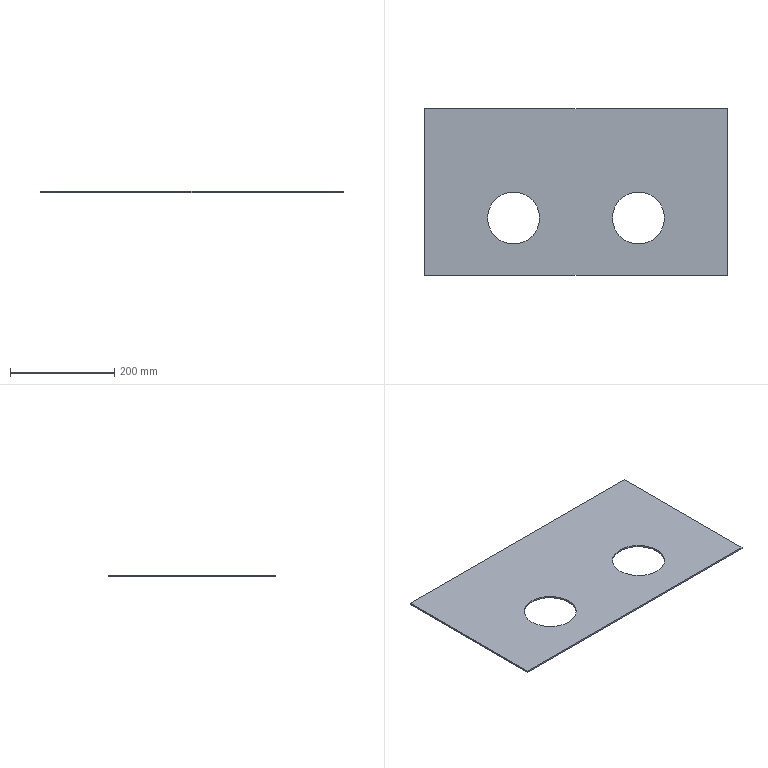Part | SolidWorks | features FlatPattern 1, SMBaseFlange 1, SheetMetal 1 | 1 solid | 10 faces | box 582 x 320 x 3 mm | volume 511596 mm3 | plane 6 | cylinder 4 | commonest cylinder face diameters 100 x4
STEP:
#1=CARTESIAN_POINT('',(69.801,-190.647,-3.));
#2=VERTEX_POINT('',#1);
#3=CARTESIAN_POINT('',(169.801,-190.647,-3.));
#4=VERTEX_POINT('',#3);
#5=CARTESIAN_POINT('',(119.801,-190.647,-3.));
#6=DIRECTION('',(0.,0.,1.));
#7=DIRECTION('',(1.,0.,0.));
#8=AXIS2_PLACEMENT_3D('',#5,#6,#7);
#9=CIRCLE('',#8,50.);
#10=EDGE_CURVE('',#2,#4,#9,.T.);
#11=ORIENTED_EDGE('',*,*,#10,.F.);
#12=CARTESIAN_POINT('',(69.801,-190.647,0.));
#13=VERTEX_POINT('',#12);
#14=CARTESIAN_POINT('',(69.801,-190.647,-3.));
#15=DIRECTION('',(0.,0.,1.));
#16=VECTOR('',#15,1000.);
#17=LINE('',#14,#16);
#18=EDGE_CURVE('',#2,#13,#17,.T.);
#19=ORIENTED_EDGE('',*,*,#18,.T.);
#20=CARTESIAN_POINT('',(169.801,-190.647,0.));
#21=VERTEX_POINT('',#20);
#22=CARTESIAN_POINT('',(119.801,-190.647,0.));
#23=DIRECTION('',(0.,0.,1.));
#24=DIRECTION('',(1.,0.,0.));
#25=AXIS2_PLACEMENT_3D('',#22,#23,#24);
#26=CIRCLE('',#25,50.);
#27=EDGE_CURVE('',#13,#21,#26,.T.);
#28=ORIENTED_EDGE('',*,*,#27,.T.);
#29=CARTESIAN_POINT('',(169.801,-190.647,-3.));
#30=DIRECTION('',(0.,0.,1.));
#31=VECTOR('',#30,1000.);
#32=LINE('',#29,#31);
#33=EDGE_CURVE('',#4,#21,#32,.T.);
#34=ORIENTED_EDGE('',*,*,#33,.F.);
#35=EDGE_LOOP('',(#11,#19,#28,#34));
#36=FACE_OUTER_BOUND('',#35,.T.);
#37=CARTESIAN_POINT('',(119.801,-190.647,-3.));
#38=DIRECTION('',(0.,0.,1.));
#39=DIRECTION('',(1.,0.,0.));
#40=AXIS2_PLACEMENT_3D('',#37,#38,#39);
#41=CYLINDRICAL_SURFACE('',#40,50.);
#42=ADVANCED_FACE('',(#36),#41,.F.);
#43=CARTESIAN_POINT('',(309.801,-190.647,-3.));
#44=VERTEX_POINT('',#43);
#45=CARTESIAN_POINT('',(409.801,-190.647,-3.));
#46=VERTEX_POINT('',#45);
#47=CARTESIAN_POINT('',(359.801,-190.647,-3.));
#48=DIRECTION('',(0.,0.,1.));
#49=DIRECTION('',(1.,0.,0.));
#50=AXIS2_PLACEMENT_3D('',#47,#48,#49);
#51=CIRCLE('',#50,50.);
#52=EDGE_CURVE('',#44,#46,#51,.T.);
#53=ORIENTED_EDGE('',*,*,#52,.F.);
#54=CARTESIAN_POINT('',(309.801,-190.647,0.));
#55=VERTEX_POINT('',#54);
#56=CARTESIAN_POINT('',(309.801,-190.647,-3.));
#57=DIRECTION('',(0.,0.,1.));
#58=VECTOR('',#57,1000.);
#59=LINE('',#56,#58);
#60=EDGE_CURVE('',#44,#55,#59,.T.);
#61=ORIENTED_EDGE('',*,*,#60,.T.);
#62=CARTESIAN_POINT('',(409.801,-190.647,0.));
#63=VERTEX_POINT('',#62);
#64=CARTESIAN_POINT('',(359.801,-190.647,0.));
#65=DIRECTION('',(0.,0.,1.));
#66=DIRECTION('',(1.,0.,0.));
#67=AXIS2_PLACEMENT_3D('',#64,#65,#66);
#68=CIRCLE('',#67,50.);
#69=EDGE_CURVE('',#55,#63,#68,.T.);
#70=ORIENTED_EDGE('',*,*,#69,.T.);
#71=CARTESIAN_POINT('',(409.801,-190.647,-3.));
#72=DIRECTION('',(0.,0.,1.));
#73=VECTOR('',#72,1000.);
#74=LINE('',#71,#73);
#75=EDGE_CURVE('',#46,#63,#74,.T.);
#76=ORIENTED_EDGE('',*,*,#75,.F.);
#77=EDGE_LOOP('',(#53,#61,#70,#76));
#78=FACE_OUTER_BOUND('',#77,.T.);
#79=CARTESIAN_POINT('',(359.801,-190.647,-3.));
#80=DIRECTION('',(0.,0.,1.));
#81=DIRECTION('',(1.,0.,0.));
#82=AXIS2_PLACEMENT_3D('',#79,#80,#81);
#83=CYLINDRICAL_SURFACE('',#82,50.);
#84=ADVANCED_FACE('',(#78),#83,.F.);
#85=CARTESIAN_POINT('',(-51.199,-300.647,0.));
#86=VERTEX_POINT('',#85);
#87=CARTESIAN_POINT('',(530.801,-300.647,0.));
#88=VERTEX_POINT('',#87);
#89=CARTESIAN_POINT('',(-51.199,-300.647,0.));
#90=DIRECTION('',(1.,0.,0.));
#91=VECTOR('',#90,1000.);
#92=LINE('',#89,#91);
#93=EDGE_CURVE('',#86,#88,#92,.T.);
#94=ORIENTED_EDGE('',*,*,#93,.F.);
#95=CARTESIAN_POINT('',(-51.199,-300.647,-3.));
#96=VERTEX_POINT('',#95);
#97=CARTESIAN_POINT('',(-51.199,-300.647,-3.));
#98=DIRECTION('',(0.,0.,1.));
#99=VECTOR('',#98,1000.);
#100=LINE('',#97,#99);
#101=EDGE_CURVE('',#96,#86,#100,.T.);
#102=ORIENTED_EDGE('',*,*,#101,.F.);
#103=CARTESIAN_POINT('',(530.801,-300.647,-3.));
#104=VERTEX_POINT('',#103);
#105=CARTESIAN_POINT('',(-51.199,-300.647,-3.));
#106=DIRECTION('',(1.,0.,0.));
#107=VECTOR('',#106,1000.);
#108=LINE('',#105,#107);
#109=EDGE_CURVE('',#96,#104,#108,.T.);
#110=ORIENTED_EDGE('',*,*,#109,.T.);
#111=CARTESIAN_POINT('',(530.801,-300.647,-3.));
#112=DIRECTION('',(0.,0.,1.));
#113=VECTOR('',#112,1000.);
#114=LINE('',#111,#113);
#115=EDGE_CURVE('',#104,#88,#114,.T.);
#116=ORIENTED_EDGE('',*,*,#115,.T.);
#117=EDGE_LOOP('',(#94,#102,#110,#116));
#118=FACE_OUTER_BOUND('',#117,.T.);
#119=CARTESIAN_POINT('',(-51.199,-300.647,-3.));
#120=DIRECTION('',(0.,-1.,0.));
#121=DIRECTION('',(1.,0.,0.));
#122=AXIS2_PLACEMENT_3D('',#119,#120,#121);
#123=PLANE('',#122);
#124=ADVANCED_FACE('',(#118),#123,.T.);
#125=CARTESIAN_POINT('',(-51.199,19.353,0.));
#126=VERTEX_POINT('',#125);
#127=CARTESIAN_POINT('',(-51.199,-300.647,0.));
#128=DIRECTION('',(0.,-1.,0.));
#129=VECTOR('',#128,1000.);
#130=LINE('',#127,#129);
#131=EDGE_CURVE('',#126,#86,#130,.T.);
#132=ORIENTED_EDGE('',*,*,#131,.F.);
#133=CARTESIAN_POINT('',(-51.199,19.353,-3.));
#134=VERTEX_POINT('',#133);
#135=CARTESIAN_POINT('',(-51.199,19.353,-3.));
#136=DIRECTION('',(0.,0.,1.));
#137=VECTOR('',#136,1000.);
#138=LINE('',#135,#137);
#139=EDGE_CURVE('',#134,#126,#138,.T.);
#140=ORIENTED_EDGE('',*,*,#139,.F.);
#141=CARTESIAN_POINT('',(-51.199,-300.647,-3.));
#142=DIRECTION('',(0.,-1.,0.));
#143=VECTOR('',#142,1000.);
#144=LINE('',#141,#143);
#145=EDGE_CURVE('',#134,#96,#144,.T.);
#146=ORIENTED_EDGE('',*,*,#145,.T.);
#147=ORIENTED_EDGE('',*,*,#101,.T.);
#148=EDGE_LOOP('',(#132,#140,#146,#147));
#149=FACE_OUTER_BOUND('',#148,.T.);
#150=CARTESIAN_POINT('',(-51.199,-300.647,-3.));
#151=DIRECTION('',(-1.,0.,0.));
#152=DIRECTION('',(0.,-1.,0.));
#153=AXIS2_PLACEMENT_3D('',#150,#151,#152);
#154=PLANE('',#153);
#155=ADVANCED_FACE('',(#149),#154,.T.);
#156=CARTESIAN_POINT('',(530.801,19.353,0.));
#157=VERTEX_POINT('',#156);
#158=CARTESIAN_POINT('',(-51.199,19.353,0.));
#159=DIRECTION('',(-1.,0.,0.));
#160=VECTOR('',#159,1000.);
#161=LINE('',#158,#160);
#162=EDGE_CURVE('',#157,#126,#161,.T.);
#163=ORIENTED_EDGE('',*,*,#162,.F.);
#164=CARTESIAN_POINT('',(530.801,19.353,-3.));
#165=VERTEX_POINT('',#164);
#166=CARTESIAN_POINT('',(530.801,19.353,-3.));
#167=DIRECTION('',(0.,0.,1.));
#168=VECTOR('',#167,1000.);
#169=LINE('',#166,#168);
#170=EDGE_CURVE('',#165,#157,#169,.T.);
#171=ORIENTED_EDGE('',*,*,#170,.F.);
#172=CARTESIAN_POINT('',(-51.199,19.353,-3.));
#173=DIRECTION('',(-1.,0.,0.));
#174=VECTOR('',#173,1000.);
#175=LINE('',#172,#174);
#176=EDGE_CURVE('',#165,#134,#175,.T.);
#177=ORIENTED_EDGE('',*,*,#176,.T.);
#178=ORIENTED_EDGE('',*,*,#139,.T.);
#179=EDGE_LOOP('',(#163,#171,#177,#178));
#180=FACE_OUTER_BOUND('',#179,.T.);
#181=CARTESIAN_POINT('',(-51.199,19.353,-3.));
#182=DIRECTION('',(0.,1.,0.));
#183=DIRECTION('',(-1.,0.,0.));
#184=AXIS2_PLACEMENT_3D('',#181,#182,#183);
#185=PLANE('',#184);
#186=ADVANCED_FACE('',(#180),#185,.T.);
#187=CARTESIAN_POINT('',(530.801,19.353,0.));
#188=DIRECTION('',(0.,1.,0.));
#189=VECTOR('',#188,1000.);
#190=LINE('',#187,#189);
#191=EDGE_CURVE('',#88,#157,#190,.T.);
#192=ORIENTED_EDGE('',*,*,#191,.F.);
#193=ORIENTED_EDGE('',*,*,#115,.F.);
#194=CARTESIAN_POINT('',(530.801,19.353,-3.));
#195=DIRECTION('',(0.,1.,0.));
#196=VECTOR('',#195,1000.);
#197=LINE('',#194,#196);
#198=EDGE_CURVE('',#104,#165,#197,.T.);
#199=ORIENTED_EDGE('',*,*,#198,.T.);
#200=ORIENTED_EDGE('',*,*,#170,.T.);
#201=EDGE_LOOP('',(#192,#193,#199,#200));
#202=FACE_OUTER_BOUND('',#201,.T.);
#203=CARTESIAN_POINT('',(530.801,19.353,-3.));
#204=DIRECTION('',(1.,0.,0.));
#205=DIRECTION('',(0.,1.,0.));
#206=AXIS2_PLACEMENT_3D('',#203,#204,#205);
#207=PLANE('',#206);
#208=ADVANCED_FACE('',(#202),#207,.T.);
#209=CARTESIAN_POINT('',(119.801,-190.647,-3.));
#210=DIRECTION('',(0.,0.,1.));
#211=DIRECTION('',(1.,0.,0.));
#212=AXIS2_PLACEMENT_3D('',#209,#210,#211);
#213=CIRCLE('',#212,50.);
#214=EDGE_CURVE('',#4,#2,#213,.T.);
#215=ORIENTED_EDGE('',*,*,#214,.T.);
#216=ORIENTED_EDGE('',*,*,#10,.T.);
#217=EDGE_LOOP('',(#215,#216));
#218=FACE_BOUND('',#217,.T.);
#219=CARTESIAN_POINT('',(359.801,-190.647,-3.));
#220=DIRECTION('',(0.,0.,1.));
#221=DIRECTION('',(1.,0.,0.));
#222=AXIS2_PLACEMENT_3D('',#219,#220,#221);
#223=CIRCLE('',#222,50.);
#224=EDGE_CURVE('',#46,#44,#223,.T.);
#225=ORIENTED_EDGE('',*,*,#224,.T.);
#226=ORIENTED_EDGE('',*,*,#52,.T.);
#227=EDGE_LOOP('',(#225,#226));
#228=FACE_BOUND('',#227,.T.);
#229=ORIENTED_EDGE('',*,*,#109,.F.);
#230=ORIENTED_EDGE('',*,*,#145,.F.);
#231=ORIENTED_EDGE('',*,*,#176,.F.);
#232=ORIENTED_EDGE('',*,*,#198,.F.);
#233=EDGE_LOOP('',(#229,#230,#231,#232));
#234=FACE_OUTER_BOUND('',#233,.T.);
#235=CARTESIAN_POINT('',(0.,0.,-3.));
#236=DIRECTION('',(0.,0.,-1.));
#237=DIRECTION('',(-1.,0.,0.));
#238=AXIS2_PLACEMENT_3D('',#235,#236,#237);
#239=PLANE('',#238);
#240=ADVANCED_FACE('',(#218,#228,#234),#239,.T.);
#241=CARTESIAN_POINT('',(119.801,-190.647,0.));
#242=DIRECTION('',(0.,0.,1.));
#243=DIRECTION('',(1.,0.,0.));
#244=AXIS2_PLACEMENT_3D('',#241,#242,#243);
#245=CIRCLE('',#244,50.);
#246=EDGE_CURVE('',#21,#13,#245,.T.);
#247=ORIENTED_EDGE('',*,*,#246,.F.);
#248=ORIENTED_EDGE('',*,*,#27,.F.);
#249=EDGE_LOOP('',(#247,#248));
#250=FACE_BOUND('',#249,.T.);
#251=CARTESIAN_POINT('',(359.801,-190.647,0.));
#252=DIRECTION('',(0.,0.,1.));
#253=DIRECTION('',(1.,0.,0.));
#254=AXIS2_PLACEMENT_3D('',#251,#252,#253);
#255=CIRCLE('',#254,50.);
#256=EDGE_CURVE('',#63,#55,#255,.T.);
#257=ORIENTED_EDGE('',*,*,#256,.F.);
#258=ORIENTED_EDGE('',*,*,#69,.F.);
#259=EDGE_LOOP('',(#257,#258));
#260=FACE_BOUND('',#259,.T.);
#261=ORIENTED_EDGE('',*,*,#93,.T.);
#262=ORIENTED_EDGE('',*,*,#191,.T.);
#263=ORIENTED_EDGE('',*,*,#162,.T.);
#264=ORIENTED_EDGE('',*,*,#131,.T.);
#265=EDGE_LOOP('',(#261,#262,#263,#264));
#266=FACE_OUTER_BOUND('',#265,.T.);
#267=CARTESIAN_POINT('',(0.,0.,0.));
#268=DIRECTION('',(0.,0.,-1.));
#269=DIRECTION('',(-1.,0.,0.));
#270=AXIS2_PLACEMENT_3D('',#267,#268,#269);
#271=PLANE('',#270);
#272=ADVANCED_FACE('',(#250,#260,#266),#271,.F.);
#273=ORIENTED_EDGE('',*,*,#60,.F.);
#274=ORIENTED_EDGE('',*,*,#224,.F.);
#275=ORIENTED_EDGE('',*,*,#75,.T.);
#276=ORIENTED_EDGE('',*,*,#256,.T.);
#277=EDGE_LOOP('',(#273,#274,#275,#276));
#278=FACE_OUTER_BOUND('',#277,.T.);
#279=CARTESIAN_POINT('',(359.801,-190.647,-3.));
#280=DIRECTION('',(0.,0.,1.));
#281=DIRECTION('',(1.,0.,0.));
#282=AXIS2_PLACEMENT_3D('',#279,#280,#281);
#283=CYLINDRICAL_SURFACE('',#282,50.);
#284=ADVANCED_FACE('',(#278),#283,.F.);
#285=ORIENTED_EDGE('',*,*,#18,.F.);
#286=ORIENTED_EDGE('',*,*,#214,.F.);
#287=ORIENTED_EDGE('',*,*,#33,.T.);
#288=ORIENTED_EDGE('',*,*,#246,.T.);
#289=EDGE_LOOP('',(#285,#286,#287,#288));
#290=FACE_OUTER_BOUND('',#289,.T.);
#291=CARTESIAN_POINT('',(119.801,-190.647,-3.));
#292=DIRECTION('',(0.,0.,1.));
#293=DIRECTION('',(1.,0.,0.));
#294=AXIS2_PLACEMENT_3D('',#291,#292,#293);
#295=CYLINDRICAL_SURFACE('',#294,50.);
#296=ADVANCED_FACE('',(#290),#295,.F.);
#297=CLOSED_SHELL('',(#42,#84,#124,#155,#186,#208,#240,#272,#284,#296));
#298=MANIFOLD_SOLID_BREP('',#297);
#299=CARTESIAN_POINT('',(0.,0.,0.));
#300=DIRECTION('',(0.,0.,1.));
#301=DIRECTION('',(1.,0.,0.));
#302=AXIS2_PLACEMENT_3D('',#299,#300,#301);
#303=(LENGTH_UNIT()NAMED_UNIT(*)SI_UNIT(.MILLI.,.METRE.));
#304=UNCERTAINTY_MEASURE_WITH_UNIT(LENGTH_MEASURE(0.00001),#303,'','');
#305=(NAMED_UNIT(*)PLANE_ANGLE_UNIT()SI_UNIT($,.RADIAN.));
#306=(NAMED_UNIT(*)SI_UNIT($,.STERADIAN.)SOLID_ANGLE_UNIT());
#307=(GEOMETRIC_REPRESENTATION_CONTEXT(3)GLOBAL_UNCERTAINTY_ASSIGNED_CONTEXT((#304))GLOBAL_UNIT_ASSIGNED_CONTEXT((#303,#305,#306))REPRESENTATION_CONTEXT('',''));
#308=ADVANCED_BREP_SHAPE_REPRESENTATION('',(#298,#302),#307);